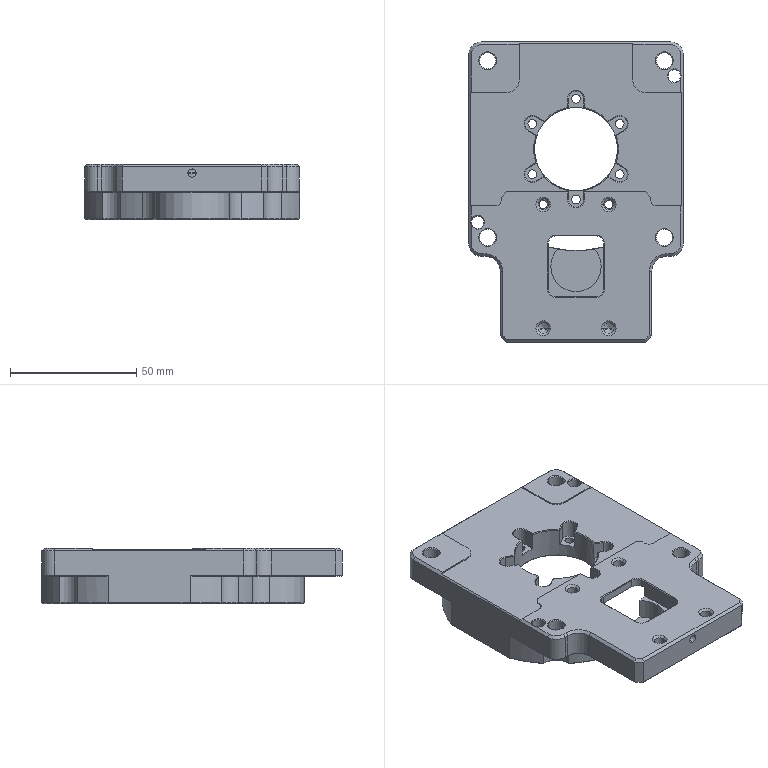Part | SolidWorks | features BaseBody 1 | 1 solid | 305 faces | box 85 x 119 x 22 mm | volume 77366 mm3 | cone 110 | plane 94 | cylinder 92 | torus 9 | commonest cylinder face diameters 3.5 x12 6 x12 4.2 x8 6.5 x8 91 x8 5 x6